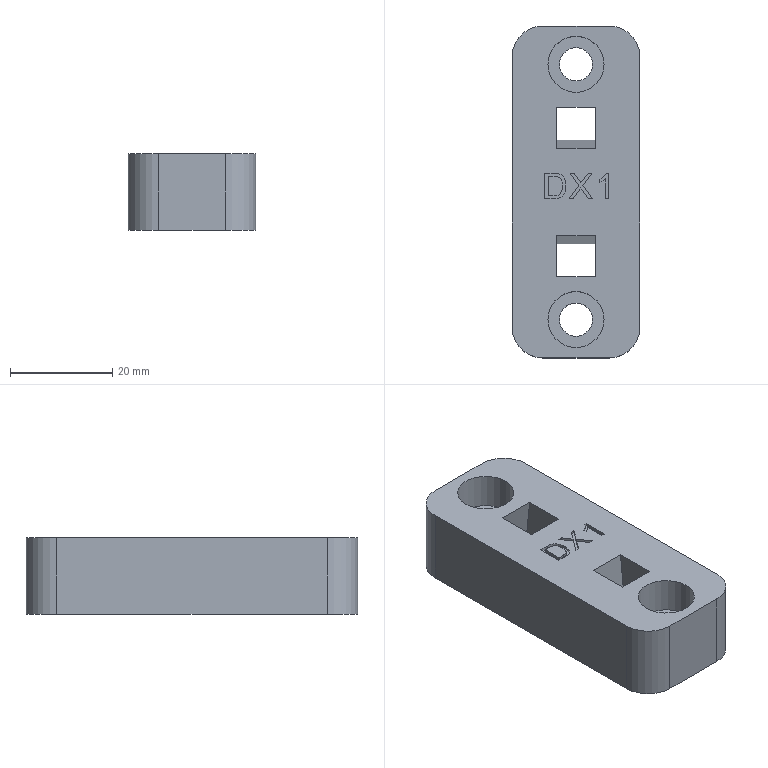Part | STEP file | solid 107 | 1 solid | 55 faces | box 25 x 65 x 15 mm | volume 20230 mm3 | plane 43 | cylinder 8 | other 4 | commonest cylinder face diameters 12 x4 6.5 x2 11 x2